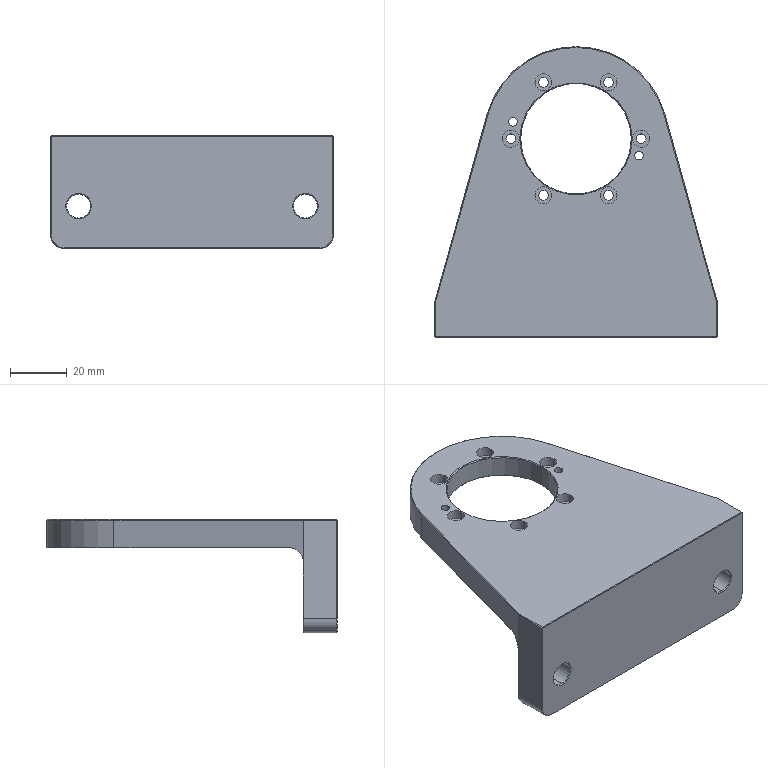NC program | NX | posted with a generic post | part box 100 x 102.5 x 40 mm
Lines 1022 to 2296 of 2296:
(ZLEVEL_PROFILE_1 , TOOL : D6R0.5)
N2006 T16 M6
N2008 G54
N2010 G17 G0 G90 X53.141 Y-17.388 B0. C0. S9500 M3
N2012 G43 Z30. H16
N2014 Z-22.1
N2016 G94 G1 Z-25.1 F3500.
N2018 G3 X50.204 Y-15. R3.
N2020 G1 X-50.204
N2022 X-50.214 Z-25.2
N2024 X50.214
N2026 X50.225 Z-25.3
N2028 X-50.225
N2030 X-50.236 Y-15.001 Z-25.4
N2032 X50.236
N2034 X50.247 Y-15.002 Z-25.5
N2036 X-50.247
N2038 X-50.258 Y-15.004 Z-25.6
N2040 X-49.999 Y-15.001
N2042 X49.999
N2044 X50.258 Y-15.004
N2046 X50.268 Y-15.01 Z-25.7
N2048 X49.998 Y-15.004
N2050 X-49.998
N2052 X-50.268 Y-15.01
N2054 X-50.278 Y-15.016 Z-25.8
N2056 X-49.997 Y-15.01
N2058 X49.997
N2060 X50.278 Y-15.016
N2062 X50.289 Y-15.024 Z-25.899
N2064 X49.994 Y-15.018
N2066 X-49.994
N2068 X-50.289 Y-15.024
N2070 X-50.3 Y-15.031 Z-25.999
N2072 X-49.991 Y-15.028
N2074 X49.991
N2076 X50.3 Y-15.031
N2078 X50.312 Y-15.043 Z-26.098
N2080 X49.987 Y-15.04
N2082 X-49.987
N2084 X-50.312 Y-15.043
N2086 X-50.323 Y-15.059 Z-26.197
N2088 X-49.982 Y-15.054
N2090 X49.982
N2092 X50.323 Y-15.059
N2094 X50.334 Y-15.076 Z-26.296
N2096 X49.978 Y-15.071
N2098 X-49.978
N2100 X-50.334 Y-15.076
N2102 X-50.344 Y-15.095 Z-26.394
N2104 X-49.972 Y-15.09
N2106 X49.972
N2108 X50.344 Y-15.095
N2110 X50.354 Y-15.114 Z-26.492
N2112 X49.965 Y-15.111
N2114 X-49.965
N2116 X-50.354 Y-15.114
N2118 X-50.365 Y-15.137 Z-26.589
N2120 X-49.958 Y-15.134
N2122 X49.958
N2124 X50.365 Y-15.137
N2126 X50.375 Y-15.164 Z-26.686
N2128 X49.95 Y-15.159
N2130 X-49.95
N2132 X-50.375 Y-15.164
N2134 X-50.385 Y-15.191 Z-26.782
N2136 G3 X-49.942 Y-15.186 R21.556
N2138 G1 X49.942
N2140 G3 X50.385 Y-15.191 R4.196
N2142 G1 X50.396 Y-15.221 Z-26.877
N2144 G2 X49.932 Y-15.216 R5.14
N2146 G1 X-49.932
N2148 G2 X-50.396 Y-15.221 R30.468
N2150 G1 X-50.406 Y-15.251 Z-26.972
N2152 X-49.922 Y-15.248
N2154 X49.922
N2156 X50.406 Y-15.251
N2158 X50.405 Y-15.267 Z-27.019
N2160 X50.403 Y-15.285 Z-27.066
N2162 X49.912 Y-15.281
N2164 X-49.912
N2166 X-50.403 Y-15.285
N2168 X-50.39 Y-15.324 Z-27.159
N2170 X-49.901 Y-15.317
N2172 X49.901
N2174 X50.39 Y-15.324
N2176 X50.377 Y-15.362 Z-27.252
N2178 X49.868 Y-15.355
N2180 X-49.868
N2182 X-50.377 Y-15.362
N2184 X-50.364 Y-15.4 Z-27.344
N2186 X-49.877 Y-15.395
N2188 X49.877
N2190 X50.364 Y-15.4
N2192 X50.351 Y-15.438 Z-27.434
N2194 X49.863 Y-15.437
N2196 X-49.863
N2198 X-50.351 Y-15.438
N2200 X-50.345 Y-15.462 Z-27.479
N2202 X-50.339 Y-15.485 Z-27.524
N2204 X-49.85 Y-15.481
N2206 X49.85
N2208 X50.339 Y-15.485
N2210 X50.333 Y-15.508 Z-27.568
N2212 X50.326 Y-15.532 Z-27.613
N2214 X49.836 Y-15.527
N2216 X-49.836
N2218 X-50.326 Y-15.532
N2220 X-50.314 Y-15.578 Z-27.7
N2222 X-49.821 Y-15.575
N2224 X49.821
N2226 X50.314 Y-15.578
N2228 X50.3 Y-15.626 Z-27.787
N2230 X49.847 Y-15.628
N2232 X49.805 Y-15.624
N2234 X-49.805
N2236 X-49.847 Y-15.628
N2238 X-50.3 Y-15.626
N2240 X-50.282 Y-15.68 Z-27.872
N2242 X-49.847 Y-15.682
N2244 X-49.789 Y-15.676
N2246 X49.789
N2248 X49.847 Y-15.682
N2250 X50.283 Y-15.68
N2252 X50.265 Y-15.733 Z-27.957
N2254 X50.193 Y-15.735
N2256 X49.847 Y-15.734
N2258 X49.772 Y-15.73
N2260 X-49.772
N2262 X-49.847 Y-15.734
N2264 X-50.193 Y-15.735
N2266 X-50.265 Y-15.733
N2268 X-50.248 Y-15.786 Z-28.04
N2270 X-50.193 Y-15.788
N2272 X-49.755 Y-15.785
N2274 X49.755
N2276 X50.193 Y-15.788
N2278 X50.248 Y-15.786
N2280 X50.232 Y-15.846 Z-28.122
N2282 X50.193 Y-15.848
N2284 X49.737 Y-15.843
N2286 X-49.737
N2288 X-50.193 Y-15.848
N2290 X-50.232 Y-15.846
N2292 X-50.216 Y-15.905 Z-28.202
N2294 X-49.719 Y-15.902
N2296 X49.719
N2298 X50.216 Y-15.905
N2300 X50.199 Y-15.965 Z-28.281
N2302 X49.7 Y-15.962
N2304 X-49.7
N2306 X-50.199 Y-15.965
N2308 X-50.179 Y-16.032 Z-28.359
N2310 X-49.681 Y-16.025
N2312 X49.681
N2314 X50.179 Y-16.032
N2316 X50.159 Y-16.099 Z-28.436
N2318 X49.661 Y-16.089
N2320 X-49.661
N2322 X-50.158 Y-16.099
N2324 X-50.138 Y-16.164 Z-28.511
N2326 X-49.64 Y-16.155
N2328 X49.64
N2330 X50.138 Y-16.165
N2332 X50.119 Y-16.23 Z-28.584
N2334 X49.619 Y-16.223
N2336 X-49.619
N2338 X-50.119 Y-16.23
N2340 X-50.099 Y-16.295 Z-28.656
N2342 X-49.598 Y-16.292
N2344 X49.598
N2346 X50.099 Y-16.295
N2348 X50.076 Y-16.371 Z-28.726
N2350 X49.575 Y-16.37
N2352 X49.562 Y-16.363
N2354 X-49.562
N2356 X-49.575 Y-16.37
N2358 X-50.076 Y-16.371
N2360 X-50.053 Y-16.446 Z-28.795
N2362 X-49.539 Y-16.435
N2364 X49.539
N2366 X50.053 Y-16.446
N2368 X50.031 Y-16.519 Z-28.862
N2370 X49.516 Y-16.509
N2372 X-49.516
N2374 X-50.031 Y-16.519
N2376 X-50.009 Y-16.591 Z-28.928
N2378 X-49.507 Y-16.584
N2380 X49.507
N2382 X50.009 Y-16.591
N2384 X49.986 Y-16.665 Z-28.991
N2386 X49.483 Y-16.667
N2388 X49.469 Y-16.661
N2390 X-49.469
N2392 X-49.483 Y-16.667
N2394 X-49.986 Y-16.665
N2396 X-49.961 Y-16.748 Z-29.053
N2398 X-49.5 Y-16.75
N2400 X-49.444 Y-16.739
N2402 X49.444
N2404 X49.5 Y-16.75
N2406 X49.961 Y-16.748
N2408 X49.936 Y-16.828 Z-29.114
N2410 X49.5 Y-16.83
N2412 X49.42 Y-16.818
N2414 X-49.42
N2416 X-49.5 Y-16.83
N2418 X-49.936 Y-16.828
N2420 X-49.913 Y-16.907 Z-29.172
N2422 X-49.394 Y-16.899
N2424 X49.394
N2426 X49.913 Y-16.907
N2428 X49.89 Y-16.984 Z-29.229
N2430 X49.383 Y-16.981
N2432 X-49.383
N2434 X-49.89 Y-16.984
N2436 X-49.864 Y-17.069 Z-29.284
N2438 X-49.34 Y-17.064
N2440 X49.34
N2442 X49.864 Y-17.069
N2444 X49.838 Y-17.155 Z-29.336
N2446 X49.314 Y-17.148
N2448 X-49.314
N2450 X-49.838 Y-17.155
N2452 X-49.811 Y-17.242 Z-29.388
N2454 X-49.287 Y-17.233
N2456 X49.287
N2458 X49.811 Y-17.242
N2460 X49.785 Y-17.326 Z-29.437
N2462 X49.294 Y-17.325
N2464 X49.278 Y-17.32
N2466 X-49.278
N2468 X-49.295 Y-17.325
N2470 X-49.785 Y-17.326
N2472 X-49.757 Y-17.419 Z-29.484
N2474 X-49.242 Y-17.407
N2476 X49.242
N2478 X49.757 Y-17.419
N2480 X49.729 Y-17.509 Z-29.529
N2482 X49.214 Y-17.496
N2484 X-49.214
N2486 X-49.729 Y-17.509
N2488 X-49.703 Y-17.594 Z-29.572
N2490 X-49.186 Y-17.585
N2492 X49.186
N2494 X49.703 Y-17.594
N2496 X49.677 Y-17.678 Z-29.613
N2498 X49.167 Y-17.675
N2500 X-49.167
N2502 X-49.677 Y-17.678
N2504 X-49.647 Y-17.778 Z-29.653
N2506 X-49.139 Y-17.766
N2508 X49.139
N2510 X49.647 Y-17.778
N2512 X49.618 Y-17.872 Z-29.69
N2514 X49.154
N2516 X49.11 Y-17.858
N2518 X-49.11
N2520 X-49.154 Y-17.872
N2522 X-49.618
N2524 X-49.591 Y-17.961 Z-29.725
N2526 X-49.154 Y-17.962
N2528 X-49.082 Y-17.95
N2530 X49.082
N2532 X49.154 Y-17.962
N2534 X49.59
N2536 X49.562 Y-18.054 Z-29.758
N2538 X49.035 Y-18.043
N2540 X-49.035
N2542 X-49.562 Y-18.054
N2544 X-49.533 Y-18.152 Z-29.788
N2546 X-49.005 Y-18.136
N2548 X49.005
N2550 X49.533 Y-18.152
N2552 X49.505 Y-18.243 Z-29.817
N2554 X48.976 Y-18.23
N2556 X-48.976
N2558 X-49.505 Y-18.243
N2560 X-49.477 Y-18.336 Z-29.844
N2562 X-48.947 Y-18.324
N2564 X48.947
N2566 X49.477 Y-18.336
N2568 X49.445 Y-18.439 Z-29.868
N2570 X48.92 Y-18.418
N2572 X-48.92
N2574 X-49.445 Y-18.439
N2576 X-49.414 Y-18.537 Z-29.89
N2578 X-48.891 Y-18.513
N2580 X48.891
N2582 X49.415 Y-18.538
N2584 X49.387 Y-18.627 Z-29.911
N2586 X48.861 Y-18.607
N2588 X-48.861
N2590 X-49.387 Y-18.626
N2592 X-49.361 Y-18.711 Z-29.929
N2594 X-48.848 Y-18.701
N2596 X48.848
N2598 X49.361 Y-18.712
N2600 X49.313 Y-18.868 Z-29.95
N2602 X48.799 Y-18.831
N2604 X-48.799
N2606 X-49.313 Y-18.868
N2608 G3 X-52.015 Y-21.161 R3.
N2610 G1 Z-26.95
N2612 G0 Z30.
(ZLEVEL_PROFILE_1_COPY , TOOL : D6R0.5)
N2614 X49.554 Y3.375
N2616 Z2.995
N2618 G1 Z-0.005
N2620 G3 X47.672 Y0.227 R3.
N2622 G1 X47.734 Y-0.3
N2624 Y-12.
N2626 X47.667 Y-12.512
N2628 X47.776 Y-12.502 Z-0.01
N2630 X47.832 Y-12.
N2632 Y-0.3
N2634 X47.777 Y0.203
N2636 X47.831 Y0.222 Z-0.014
N2638 X47.851 Y0.23 Z-0.017
N2640 X47.858 Y0.197
N2642 X47.934 Y-0.3
N2644 Y-12.
N2646 X47.852 Y-12.525
N2648 X47.913 Y-12.544 Z-0.02
N2650 X47.923 Y-12.547 Z-0.024
N2652 X48.011 Y-12.
N2654 Y-0.3
N2656 X47.918 Y0.255
N2658 X47.977 Y0.277 Z-0.027
N2660 X47.98 Y0.278 Z-0.03
N2662 X48.003 Y0.197
N2664 X48.075 Y-0.3
N2666 Y-12.
N2668 X47.989 Y-12.568
N2670 X48.038 Y-12.583 Z-0.034
N2672 X48.061 Y-12.59 Z-0.037
N2674 X48.138 Y-12.
N2676 Y-0.3
N2678 G3 X48.047 Y0.303 R2.011
N2680 G1 X48.134 Y0.288 Z-0.046
N2682 X48.153 Y0.197
N2684 X48.21 Y-0.3
N2686 Y-12.
N2688 X48.138 Y-12.6
N2690 X48.104 Y-12.71
N2692 X48.223 Y-12.597 Z-0.058
N2694 X48.294 Y-12.
N2696 Y-0.3
N2698 X48.188 Y0.369
N2700 X48.252 Z-0.065
N2702 X48.277 Z-0.072
N2704 X48.388 Y-0.3
N2706 Y-12.
N2708 X48.322 Y-12.559
N2710 X48.427 Y-12.513 Z-0.089
N2712 X48.484 Y-12.
N2714 Y-0.3
N2716 X48.38 Y0.369
N2718 X48.46 Y0.3 Z-0.098
N2720 X48.518 Y0.227 Z-0.107
N2722 X48.58 Y-0.3
N2724 Y-12.
N2726 X48.517 Y-12.532
N2728 X48.607 Y-12.581 Z-0.127
N2730 X48.676 Y-12.
N2732 Y-0.3
N2734 X48.615 Y0.197
N2736 X48.599 Y0.268
N2738 X48.64 Y0.288 Z-0.134
N2740 X48.654 Y0.295 Z-0.141
N2742 X48.679 Y0.197
N2744 X48.738 Y-0.3
N2746 Y-12.
N2748 X48.663 Y-12.613
N2750 X48.7 Y-12.636 Z-0.151
N2752 X48.729 Y-12.654 Z-0.161
N2754 X48.747 Y-12.6
N2756 X48.819 Y-12.
N2758 Y-0.3
N2760 X48.731 Y0.334
N2762 X48.703 Y0.466
N2764 X48.68 Y0.542
N2766 X48.764 Y0.432 Z-0.173
N2768 X48.835 Y0.318 Z-0.185
N2770 X48.861 Y0.197
N2772 X48.914 Y-0.3
N2774 Y-12.
N2776 X48.845 Y-12.6
N2778 X48.839 Y-12.62
N2780 X48.938 Y-12.57 Z-0.211
N2782 X49.009 Y-12.
N2784 Y-0.3
N2786 X48.908 Y0.369
N2788 X48.97 Z-0.225
N2790 X49.002 Z-0.239
N2792 X49.103 Y-0.3
N2794 Y-12.
N2796 X49.037 Y-12.536
N2798 X49.148 Y-12.502 Z-0.268
N2800 X49.164 Y-12.416
N2802 X49.197 Y-12.
N2804 Y-0.3
N2806 X49.101 Y0.369
N2808 X49.178 Y0.286 Z-0.284
N2810 X49.236 Y0.2 Z-0.3
N2812 X49.291 Y-0.3
N2814 Y-12.
N2816 X49.254 Y-12.429
N2818 X49.24 Y-12.509
N2820 X49.282 Y-12.6 Z-0.321
N2822 X49.299 Y-12.523
N2824 X49.351 Y-12.
N2826 Y-0.3
N2828 X49.295 Y0.2
N2830 X49.366 Z-0.347
N2832 X49.422 Y-0.3
N2834 Y-12.
N2836 X49.353 Y-12.601
N2838 X49.399 Z-0.364
N2840 X49.446 Y-12.6 Z-0.382
N2842 X49.514 Y-12.
N2844 Y-0.3
N2846 X49.464 Y0.2
N2848 X49.512 Z-0.4
N2850 X49.554 Z-0.419
N2852 X49.605 Y-0.3
N2854 Y-12.
N2856 X49.559 Y-12.498
N2858 X49.556 Y-12.504
N2860 X49.646 Y-12.5 Z-0.458
N2862 X49.656 Y-12.458
N2864 X49.696 Y-12.
N2866 Y-0.3
N2868 X49.642 Y0.2
N2870 X49.694 Z-0.478
N2872 X49.733 Z-0.498
N2874 X49.786 Y-0.3
N2876 Y-12.
N2878 X49.744 Y-12.475
N2880 X49.737 Y-12.5
N2882 X49.829 Z-0.54
N2884 X49.831 Y-12.491
N2886 X49.876 Y-12.
N2888 Y-0.3
N2890 X49.828 Y0.2
N2892 X49.874 Z-0.561
N2894 X49.914 Z-0.583
N2896 X49.965 Y-0.3
N2898 Y-12.
N2900 X49.92 Y-12.427
N2902 X49.975 Z-0.606
N2904 X50.006 Z-0.628
N2906 X50.053 Y-12.
N2908 Y-0.3
N2910 X49.999 Y0.2
N2912 X50.051 Z-0.652
N2914 X50.088 Z-0.675
N2916 X50.14 Y-0.3
N2918 Y-12.
N2920 X50.095 Y-12.427
N2922 X50.175 Y-12.507 Z-0.723
N2924 X50.193 Y-12.413
N2926 X50.227 Y-12.
N2928 Y-0.3
N2930 X50.18 Y0.2
N2932 X50.223 Y0.205 Z-0.748
N2934 X50.26 Y0.209 Z-0.773
N2936 X50.312 Y-0.3
N2938 Y-12.
N2940 X50.256 Y-12.508
N2942 X50.306 Y-12.515 Z-0.799
N2944 X50.337 Y-12.519 Z-0.825
N2946 X50.397 Y-12.
N2948 Y-0.3
N2950 X50.341 Y0.22
N2952 X50.388 Y0.226 Z-0.851
N2954 X50.424 Y0.231 Z-0.878
N2956 X50.481 Y-0.3
N2958 Y-12.
N2960 X50.42 Y-12.53
N2962 X50.469 Y-12.537 Z-0.905
N2964 X50.505 Y-12.542 Z-0.932
N2966 G3 X50.563 Y-12. R3.656
N2968 G1 Y-0.3
N2970 X50.509 Y0.242
N2972 X50.55 Y0.241 Z-0.959
N2974 X50.589 Y0.24 Z-0.987
N2976 X50.644 Y-0.3
N2978 Y-12.
N2980 X50.584 Y-12.539
N2982 X50.632 Y-12.533 Z-1.016
N2984 X50.664 Y-12.529 Z-1.044
N2986 X50.725 Y-12.
N2988 Y-0.3
N2990 X50.669 Y0.229
N2992 X50.75 Y0.218 Z-1.103
N2994 X50.804 Y-0.3
N2996 Y-12.
N2998 X50.746 Y-12.517
N3000 X50.797 Y-12.51 Z-1.134
N3002 X50.829 Y-12.506 Z-1.164
N3004 G3 X50.883 Y-12. R3.548
N3006 G1 Y-0.3
N3008 X50.834 Y0.207
N3010 X50.914 Y0.2 Z-1.226
N3012 X50.961 Y-0.3
N3014 Y-12.
N3016 X50.91 Y-12.499
N3018 X50.955 Z-1.257
N3020 X50.983 Z-1.289
N3022 X51.038 Y-12.
N3024 Y-0.3
N3026 X50.987 Y0.2
N3028 X51.031 Z-1.321
N3030 X51.062 Z-1.354
N3032 X51.113 Y-0.3
N3034 Y-12.
N3036 X51.057 Y-12.499
N3038 X51.106 Z-1.387
N3040 X51.133 Z-1.42
N3042 G3 X51.188 Y-12. R3.177
N3044 G1 Y-0.3
N3046 X51.138 Y0.2
N3048 X51.18 Z-1.453
N3050 X51.216 Z-1.487
N3052 X51.261 Y-0.3
N3054 Y-12.
N3056 G2 X51.212 Y-12.499 R2.867
N3058 G1 X51.253 Z-1.521
N3060 X51.281 Z-1.556
N3062 X51.333 Y-12.
N3064 Y-0.3
N3066 X51.285 Y0.2
N3068 X51.324 Z-1.591
N3070 X51.353 Z-1.626
N3072 X51.404 Y-0.3
N3074 Y-12.
N3076 X51.35 Y-12.5
N3078 X51.394 Z-1.661
N3080 X51.42 Z-1.697
N3082 X51.473 Y-12.
N3084 Y-0.3
N3086 X51.422 Y0.2
N3088 X51.463 Z-1.733
N3090 X51.492 Z-1.77
N3092 X51.542 Y-0.3
N3094 Y-12.
N3096 G2 X51.492 Y-12.5 R3.594
N3098 G1 X51.531 Z-1.806
N3100 X51.564 Z-1.843
N3102 X51.577 Y-12.404
N3104 X51.608 Y-12.
N3106 Y-0.3
N3108 X51.564 Y0.2
N3110 X51.597 Z-1.881
N3112 X51.626 Z-1.918
N3114 X51.674 Y-0.3
N3116 Y-12.
N3118 X51.627 Y-12.5
N3120 X51.662 Z-1.957
N3122 X51.688 Z-1.995
N3124 X51.738 Y-12.
N3126 Y-0.3
N3128 X51.687 Y0.2
N3130 X51.726 Z-2.033
N3132 X51.749 Z-2.072
N3134 X51.801 Y-0.3
N3136 Y-12.
N3138 X51.749 Y-12.5
N3140 X51.789 Z-2.111
N3142 X51.812 Z-2.151
N3144 G3 X51.863 Y-12. R3.703
N3146 G1 Y-0.3
N3148 X51.812 Y0.2
N3150 X51.849 Z-2.19
N3152 X51.875 Z-2.23
N3154 G2 X51.923 Y-0.3 R5.272
N3156 G1 Y-12.
N3158 G2 X51.875 Y-12.5 R3.552
N3160 G1 X51.909 Z-2.271
N3162 X51.937 Z-2.311
N3164 G3 X51.981 Y-12. R4.011
N3166 G1 Y-0.3
N3168 G3 X51.937 Y0.2 R5.865
N3170 G1 X51.967 Z-2.352
N3172 X51.993 Z-2.393
N3174 G2 X52.038 Y-0.3 R5.372
N3176 G1 Y-12.
N3178 G2 X51.996 Y-12.501 R4.747
N3180 G1 X52.023 Z-2.434
N3182 X52.052 Z-2.476
N3184 G3 X52.094 Y-12. R4.38
N3186 G1 Y-0.3
N3188 G3 X52.049 Y0.201 R4.749
N3190 G1 X52.077 Z-2.518
N3192 X52.104 Z-2.56
N3194 G2 X52.148 Y-0.3 R4.373
N3196 G1 Y-12.
N3198 G2 X52.103 Y-12.501 R4.438
N3200 G1 X52.131 Z-2.602
N3202 X52.154 Z-2.644
N3204 G3 X52.201 Y-12. R4.542
N3206 G1 Y-0.3
N3208 G3 X52.155 Y0.201 R4.671
N3210 G1 X52.183 Z-2.687
N3212 X52.206 Y0.2 Z-2.73
N3214 G2 X52.252 Y-0.3 R5.016
N3216 G1 Y-12.
N3218 G2 X52.207 Y-12.501 R3.849
N3220 G1 X52.233 Y-12.5 Z-2.773
N3222 X52.258 Z-2.817
N3224 G3 X52.301 Y-12. R4.005
N3226 G1 Y-0.3
N3228 G3 X52.258 Y0.2 R5.42
N3230 G1 X52.282 Z-2.861
N3232 X52.304 Z-2.904
N3234 G2 X52.349 Y-0.3 R6.652
N3236 G1 Y-12.
N3238 G2 X52.307 Y-12.501 R4.563
N3240 G1 X52.33 Z-2.949
N3242 X52.356 Z-2.993
N3244 G3 X52.395 Y-12. R4.798
N3246 G1 Y-0.3
N3248 G3 X52.349 Y0.201 R6.111
N3250 G1 X52.375 Z-3.038
N3252 X52.395 Z-3.082
N3254 G2 X52.44 Y-0.3 R5.647
N3256 G1 Y-12.
N3258 G2 X52.399 Y-12.502 R4.675
N3260 G1 X52.418 Z-3.127
N3262 X52.44 Z-3.172
N3264 G3 X52.483 Y-12. R4.85
N3266 G1 Y-0.3
N3268 G3 X52.44 Y0.202 R5.245
N3270 G1 X52.461 Y0.201 Z-3.218
N3272 X52.479 Z-3.263
N3274 G2 X52.525 Y-0.3 R6.023
N3276 G1 Y-12.
N3278 G2 X52.48 Y-12.502 R4.294
N3280 G1 X52.501 Z-3.309
N3282 X52.52 Y-12.501 Z-3.355
N3284 G3 X52.564 Y-12. R4.318
N3286 G1 Y-0.3
N3288 G3 X52.517 Y0.201 R6.021
N3290 G1 X52.54 Z-3.401
N3292 X52.556 Y0.2 Z-3.447
N3294 G2 X52.603 Y-0.3 R6.017
N3296 G1 Y-12.
N3298 G2 X52.56 Y-12.501 R4.34
N3300 G1 X52.578 Z-3.494
N3302 X52.6 Z-3.54
N3304 G3 X52.639 Y-12. R5.108
N3306 G1 Y-0.3
N3308 G3 X52.595 Y0.2 R6.011
N3310 G1 X52.615 Z-3.587
N3312 X52.63 Z-3.634
N3314 X52.674 Y-0.3
N3316 Y-12.
N3318 X52.635 Y-12.501
N3320 X52.647 Z-3.681
N3322 X52.666 Z-3.728
N3324 X52.707 Y-12.
N3326 Y-0.3
N3328 X52.659 Y0.201
N3330 X52.679 Z-3.776
N3332 X52.689 Z-3.823
N3334 X52.738 Y-0.3
N3336 Y-12.
N3338 X52.696 Y-12.502
N3340 X52.709 Y-12.503 Z-3.871
N3342 X52.727 Z-3.919
N3344 X52.768 Y-12.
N3346 Y-0.3
N3348 G3 X52.719 Y0.202 R7.437
N3350 G1 X52.738 Z-3.967
N3352 X52.749 Z-4.015
N3354 G2 X52.796 Y-0.3 R2.742
N3356 G1 Y-12.
N3358 G2 X52.758 Y-12.504 R4.852
N3360 G1 X52.766 Z-4.063
N3362 X52.787 Z-4.111
N3364 X52.822 Y-12.
N3366 Y-0.3
N3368 G3 X52.779 Y0.203 R7.05
N3370 G1 X52.791 Z-4.16
N3372 X52.803 Y0.202 Z-4.208
N3374 G2 X52.846 Y-0.3 R9.347
N3376 G1 Y-12.
N3378 X52.811 Y-12.504
N3380 X52.817 Z-4.257
N3382 X52.833 Z-4.306
N3384 X52.869 Y-12.
N3386 Y-0.3
N3388 G3 X52.824 Y0.202 R3.267
N3390 G1 X52.837 Z-4.354
N3392 X52.845 Z-4.403
N3394 G2 X52.89 Y-0.3 R8.797
N3396 G1 Y-12.
N3398 G2 X52.856 Y-12.504 R5.535
N3400 G1 X52.86 Z-4.452
N3402 X52.876 Y-12.503 Z-4.501
N3404 X52.909 Y-12.
N3406 Y-0.3
N3408 X52.866 Y0.202
N3410 X52.876 Z-4.551
N3412 X52.884 Z-4.6
N3414 X52.926 Y-0.3
N3416 Y-12.
N3418 X52.897 Y-12.503
N3420 X52.902 Y-12.502 Z-4.649
N3422 X52.916 Z-4.699
N3424 X52.941 Y-12.
N3426 Y-0.3
N3428 X52.901 Y0.201
N3430 X52.913 Z-4.748
N3432 X52.918 Z-4.798
N3434 X52.955 Y-0.3
N3436 Y-12.
N3438 X52.932 Y-12.501
N3440 X52.941 Z-4.847
N3442 X52.946 Y-12.5 Z-4.897
N3444 X52.967 Y-12.
N3446 Y-0.3
N3448 G3 X52.935 Y0.2 R10.725
N3450 G1 X52.948 Z-4.947
N3452 X52.952 Z-4.997
N3454 X52.977 Y-0.3
N3456 Y-12.
N3458 X52.958 Y-12.5
N3460 X52.965 Z-5.046
N3462 X52.969 Z-5.096
N3464 X52.985 Y-12.
N3466 Y-0.3
N3468 X52.966 Y0.2
N3470 X52.975 Y0.201 Z-5.196
N3472 X52.992 Y-0.3
N3474 Y-12.
N3476 X52.977 Y-12.5
N3478 X52.983 Z-5.272
N3480 X52.995 Y-12.
N3482 Y-0.3
N3484 X52.982 Y0.201
N3486 X52.988 Z-5.348
N3488 X52.998 Y-0.3
N3490 Y-12.
N3492 X52.989 Y-12.5
N3494 X52.995 Z-5.424
N3496 X52.998 Y-12.
N3498 Y-0.3
N3500 X52.995 Y0.202
N3502 X52.997 Z-5.5
N3504 X52.999 Y-0.495
N3506 Y-11.909
N3508 X52.996 Y-12.5
N3510 G3 X55.244 Y-15.416 R3.
N3512 G1 Z-2.5
N3514 G0 Z30.
N3516 X-49.553 Y-15.71
N3518 Z2.995
N3520 G1 Z-0.005
N3522 G3 X-47.665 Y-12.511 R3.
N3524 G1 X-47.734 Y-12.
N3526 Y-0.3
N3528 X-47.666 Y0.212
N3530 X-47.724 Y0.219 Z-0.008
N3532 X-47.774 Y0.225 Z-0.01
N3534 X-47.832 Y-0.3
N3536 Y-12.
N3538 X-47.785 Y-12.438
N3540 X-47.776 Y-12.502
N3542 X-47.832 Y-12.519 Z-0.014
N3544 X-47.852 Y-12.525 Z-0.017
N3546 X-47.934 Y-12.
N3548 Y-0.3
N3550 X-47.821 Y0.369
N3552 X-47.89 Z-0.024
N3554 X-48.011 Y-0.3
N3556 Y-12.
N3558 X-47.923 Y-12.547
N3560 X-47.979 Y-12.565 Z-0.027
N3562 X-47.989 Y-12.568 Z-0.03
N3564 X-48.075 Y-12.
N3566 Y-0.3
N3568 X-47.955 Y0.369
N3570 X-48.026 Z-0.037
N3572 G3 X-48.138 Y-0.3 R1.873
N3574 G1 Y-12.
N3576 X-48.061 Y-12.59
N3578 X-48.145 Y-12.575 Z-0.046
N3580 X-48.154 Y-12.533
N3582 X-48.21 Y-12.
N3584 Y-0.3
N3586 X-48.086 Y0.455
N3588 X-48.17 Y0.441 Z-0.058
N3590 X-48.294 Y-0.3
N3592 Y-12.
N3594 X-48.235 Y-12.521
N3596 X-48.332 Y-12.476 Z-0.072
N3598 X-48.388 Y-12.
N3600 Y-0.3
N3602 X-48.284 Y0.343
N3604 X-48.365 Y0.289 Z-0.08
N3606 X-48.42 Y0.232 Z-0.089
N3608 X-48.484 Y-0.3
N3610 Y-12.
N3612 X-48.439 Y-12.46
N3614 X-48.432 Y-12.496
N3616 X-48.517 Y-12.532 Z-0.107
N3618 X-48.58 Y-12.
N3620 Y-0.3
N3622 X-48.517 Y0.231
N3624 X-48.597 Y0.278 Z-0.127
N3626 X-48.615 Y0.197
N3628 X-48.676 Y-0.3
N3630 Y-12.
N3632 X-48.607 Y-12.581
N3634 X-48.664 Y-12.61 Z-0.141
N3636 X-48.738 Y-12.
N3638 Y-0.3
N3640 X-48.679 Y0.197
N3642 X-48.651 Y0.309
N3644 X-48.675 Y0.429 Z-0.151
N3646 X-48.679 Y0.542 Z-0.161
N3648 X-48.703 Y0.466
N3650 X-48.726 Y0.353
N3652 X-48.819 Y-0.3
N3654 Y-12.
N3656 X-48.747 Y-12.6
N3658 X-48.734 Y-12.64
N3660 X-48.842 Y-12.61 Z-0.185
N3662 X-48.845 Y-12.6
N3664 X-48.914 Y-12.
N3666 Y-0.3
N3668 X-48.818 Y0.395
N3670 X-48.917 Y0.334 Z-0.211
N3672 X-49.009 Y-0.3
N3674 Y-12.
N3676 X-48.96 Y-12.427
N3678 X-49.021 Z-0.225
N3680 X-49.056 Z-0.239
N3682 X-49.103 Y-12.
N3684 Y-0.3
N3686 X-49.048 Y0.197
N3688 X-49.028 Y0.27
N3690 X-49.148 Y0.203 Z-0.268
N3692 X-49.197 Y-0.3
N3694 Y-12.
N3696 X-49.154 Y-12.476
N3698 X-49.14 Y-12.538
N3700 X-49.24 Y-12.509 Z-0.3
N3702 X-49.254 Y-12.429
N3704 X-49.291 Y-12.
N3706 Y-0.3
N3708 X-49.236 Y0.2
N3710 X-49.273 Z-0.31
N3712 X-49.295 Z-0.321
N3714 X-49.351 Y-0.3
N3716 Y-12.
N3718 X-49.299 Y-12.523
N3720 X-49.282 Y-12.6
N3722 X-49.353 Y-12.601 Z-0.347
N3724 X-49.422 Y-12.
N3726 Y-0.3
N3728 X-49.366 Y0.2
N3730 X-49.421 Z-0.364
N3732 X-49.464 Z-0.382
N3734 X-49.514 Y-0.3
N3736 Y-12.
N3738 X-49.446 Y-12.6
N3740 X-49.51 Y-12.515 Z-0.4
N3742 X-49.561 Y-12.427 Z-0.419
N3744 X-49.605 Y-12.
N3746 Y-0.3
N3748 X-49.554 Y0.2
N3750 X-49.604 Z-0.438
N3752 X-49.642 Z-0.458
N3754 X-49.696 Y-0.3
N3756 Y-12.
N3758 X-49.649 Y-12.427
N3760 X-49.707 Z-0.478
N3762 X-49.74 Z-0.498
N3764 X-49.786 Y-12.
N3766 Y-0.3
N3768 X-49.733 Y0.2
N3770 X-49.784 Z-0.519
N3772 X-49.828 Z-0.54
N3774 X-49.876 Y-0.3
N3776 Y-12.
N3778 X-49.826 Y-12.49
N3780 X-49.875 Y-12.495 Z-0.561
N3782 X-49.909 Y-12.499 Z-0.583
N3784 X-49.965 Y-12.
N3786 Y-0.3
N3788 X-49.914 Y0.2
N3790 X-49.962 Z-0.606
N3792 X-49.999 Z-0.628
N3794 X-50.053 Y-0.3
N3796 Y-12.
N3798 X-49.995 Y-12.499
N3800 X-50.05 Z-0.652
N3802 X-50.083 Z-0.675
N3804 X-50.14 Y-12.
N3806 Y-0.3
N3808 X-50.088 Y0.2
N3810 X-50.138 Z-0.699
N3812 X-50.18 Z-0.723
N3814 X-50.227 Y-0.3
N3816 Y-12.
N3818 X-50.193 Y-12.413
N3820 X-50.177 Y-12.499
N3822 X-50.223 Y-12.505 Z-0.748
N3824 X-50.256 Y-12.508 Z-0.773
N3826 X-50.312 Y-12.
N3828 Y-0.3
N3830 X-50.26 Y0.209
N3832 X-50.306 Y0.215 Z-0.799
N3834 X-50.341 Y0.22 Z-0.825
N3836 X-50.397 Y-0.3
N3838 Y-12.
N3840 X-50.337 Y-12.519
N3842 X-50.388 Y-12.526 Z-0.851
N3844 X-50.42 Y-12.53 Z-0.878
N3846 X-50.481 Y-12.
N3848 Y-0.3
N3850 X-50.424 Y0.231
N3852 X-50.469 Y0.237 Z-0.905
N3854 X-50.509 Y0.242 Z-0.932
N3856 X-50.563 Y-0.3
N3858 Y-12.
N3860 G3 X-50.505 Y-12.542 R9.321
N3862 G1 X-50.55 Y-12.54 Z-0.959
N3864 X-50.584 Y-12.539 Z-0.987
N3866 X-50.644 Y-12.
N3868 Y-0.3
N3870 X-50.589 Y0.24
N3872 X-50.632 Y0.234 Z-1.016
N3874 X-50.669 Y0.229 Z-1.044
N3876 X-50.725 Y-0.3
N3878 Y-12.
N3880 X-50.664 Y-12.528
N3882 X-50.715 Y-12.521 Z-1.074
N3884 X-50.746 Y-12.517 Z-1.103
N3886 X-50.804 Y-12.
N3888 Y-0.3
N3890 X-50.75 Y0.218
N3892 X-50.834 Y0.207 Z-1.164
N3894 X-50.883 Y-0.3
N3896 Y-12.
N3898 G3 X-50.829 Y-12.506 R12.104
N3900 G1 X-50.877 Y-12.502 Z-1.195
N3902 X-50.91 Y-12.499 Z-1.226
N3904 X-50.961 Y-12.
N3906 Y-0.3
N3908 X-50.914 Y0.2
N3910 X-50.955 Z-1.257
N3912 X-50.987 Z-1.289
N3914 X-51.038 Y-0.3
N3916 Y-12.
N3918 X-50.983 Y-12.499
N3920 X-51.031 Z-1.321
N3922 X-51.057 Z-1.354
N3924 X-51.113 Y-12.
N3926 Y-0.3
N3928 X-51.062 Y0.2
N3930 X-51.106 Z-1.387
N3932 X-51.138 Z-1.42
N3934 X-51.188 Y-0.3
N3936 Y-12.
N3938 G3 X-51.133 Y-12.499 R4.952
N3940 G1 X-51.18 Z-1.453
N3942 X-51.212 Z-1.487
N3944 G2 X-51.261 Y-12. R2.867
N3946 G1 Y-0.3
N3948 X-51.216 Y0.2
N3950 X-51.252 Z-1.521
N3952 X-51.285 Z-1.556
N3954 X-51.333 Y-0.3
N3956 Y-12.
N3958 X-51.281 Y-12.499
N3960 X-51.324 Y-12.5 Z-1.591
N3962 X-51.35 Z-1.626
N3964 X-51.404 Y-12.
N3966 Y-0.3
N3968 X-51.353 Y0.2
N3970 X-51.394 Z-1.661
N3972 X-51.422 Z-1.697
N3974 X-51.473 Y-0.3
N3976 Y-12.
N3978 X-51.42 Y-12.5
N3980 X-51.463 Z-1.733
N3982 X-51.492 Z-1.77
N3984 G2 X-51.542 Y-12. R19.188
N3986 G1 Y-0.3
N3988 X-51.492 Y0.2
N3990 X-51.531 Z-1.806
N3992 X-51.564 Z-1.843
N3994 X-51.608 Y-0.3
N3996 Y-12.
N3998 X-51.577 Y-12.404
N4000 X-51.564 Y-12.5
N4002 X-51.597 Z-1.881
N4004 X-51.627 Z-1.918
N4006 X-51.674 Y-12.
N4008 Y-0.3
N4010 X-51.626 Y0.2
N4012 X-51.662 Z-1.957
N4014 X-51.687 Z-1.995
N4016 X-51.738 Y-0.3
N4018 Y-12.
N4020 X-51.688 Y-12.5
N4022 X-51.726 Z-2.033
N4024 X-51.749 Z-2.072
N4026 X-51.801 Y-12.
N4028 Y-0.3
N4030 X-51.749 Y0.2
N4032 X-51.788 Z-2.111
N4034 X-51.812 Z-2.151
N4036 X-51.863 Y-0.3
N4038 Y-12.
N4040 G3 X-51.812 Y-12.5 R3.703
N4042 G1 X-51.849 Z-2.19
N4044 X-51.875 Z-2.23
N4046 G2 X-51.923 Y-12. R3.552
N4048 G1 Y-0.3
N4050 G2 X-51.875 Y0.2 R5.272
N4052 G1 X-51.909 Z-2.271
N4054 X-51.937 Z-2.311
N4056 G3 X-51.981 Y-0.3 R5.483
N4058 G1 Y-12.
N4060 G3 X-51.937 Y-12.5 R3.409
N4062 G1 X-51.967 Z-2.352
N4064 X-51.996 Y-12.501 Z-2.393
N4066 G2 X-52.038 Y-12. R4.401
N4068 G1 Y-0.3
N4070 G2 X-51.993 Y0.2 R5.372
N4072 G1 X-52.023 Y0.201 Z-2.434
N4074 X-52.049 Z-2.476
N4076 G3 X-52.094 Y-0.3 R4.749
N4078 G1 Y-12.
N4080 G3 X-52.052 Y-12.501 R6.692
N4082 G1 X-52.077 Z-2.518
N4084 X-52.103 Z-2.56
N4086 G2 X-52.148 Y-12. R7.244
N4088 G1 Y-0.3
N4090 G2 X-52.104 Y0.201 R4.373
N4092 G1 X-52.131 Z-2.602
N4094 X-52.155 Z-2.644
N4096 G3 X-52.201 Y-0.3 R4.671
N4098 G1 Y-12.
N4100 G3 X-52.154 Y-12.501 R4.542
N4102 G1 X-52.183 Z-2.687
N4104 X-52.207 Z-2.73
N4106 G2 X-52.252 Y-12. R3.124
N4108 G1 Y-0.3
N4110 G2 X-52.206 Y0.2 R5.016
N4112 G1 X-52.234 Z-2.773
N4114 X-52.258 Z-2.817
N4116 G3 X-52.301 Y-0.3 R5.42
N4118 G1 Y-12.
N4120 G3 X-52.258 Y-12.5 R3.627
N4122 G1 X-52.282 Z-2.861
N4124 X-52.307 Y-12.501 Z-2.904
N4126 G2 X-52.349 Y-12. R4.563
N4128 G1 Y-0.3
N4130 G2 X-52.304 Y0.2 R6.652
N4132 G1 X-52.33 Z-2.949
N4134 X-52.349 Y0.201 Z-2.993
N4136 G3 X-52.395 Y-0.3 R6.111
N4138 G1 Y-12.
N4140 G3 X-52.356 Y-12.501 R4.798
N4142 G1 X-52.374 Y-12.502 Z-3.038
N4144 X-52.399 Z-3.082
N4146 G2 X-52.44 Y-12. R8.02
N4148 G1 Y-0.3
N4150 G2 X-52.395 Y0.201 R5.647
N4152 G1 X-52.418 Z-3.127
N4154 X-52.44 Y0.202 Z-3.172
N4156 G3 X-52.483 Y-0.3 R5.245
N4158 G1 Y-12.
N4160 G3 X-52.44 Y-12.502 R8.76
N4162 G1 X-52.461 Z-3.218
N4164 X-52.48 Z-3.263
N4166 G2 X-52.525 Y-12. R9.043
N4168 G1 Y-0.3
N4170 G2 X-52.479 Y0.201 R6.03
N4172 G1 X-52.501 Z-3.309
N4174 X-52.517 Z-3.355
N4176 G3 X-52.564 Y-0.3 R6.051
N4178 G1 Y-12.
N4180 G3 X-52.52 Y-12.501 R5.368
N4182 G1 X-52.54 Z-3.401
N4184 X-52.56 Z-3.447
N4186 G2 X-52.603 Y-12. R5.525
N4188 G1 Y-0.3
N4190 G2 X-52.556 Y0.2 R6.07
N4192 G1 X-52.578 Z-3.494
N4194 X-52.595 Z-3.54
N4196 G3 X-52.639 Y-0.3 R6.087
N4198 G1 Y-12.
N4200 G3 X-52.6 Y-12.501 R5.089
N4202 G1 X-52.614 Z-3.587
N4204 X-52.635 Z-3.634
N4206 X-52.674 Y-12.
N4208 Y-0.3
N4210 X-52.63 Y0.2
N4212 X-52.647 Z-3.681
N4214 X-52.66 Y0.201 Z-3.728
N4216 X-52.707 Y-0.3
N4218 Y-12.
N4220 X-52.665 Y-12.502
N4222 X-52.679 Z-3.776
N4224 X-52.696 Z-3.823
N4226 X-52.738 Y-12.
N4228 Y-0.3
N4230 X-52.69 Y0.201
N4232 X-52.71 Z-3.871
N4234 X-52.72 Y0.202 Z-3.919
N4236 G3 X-52.768 Y-0.3 R7.841
N4238 G1 Y-12.
N4240 G3 X-52.726 Y-12.503 R8.865
N4242 G1 X-52.738 Y-12.504 Z-3.967
N4244 X-52.756 Z-4.015
N4246 G2 X-52.796 Y-12. R7.511
N4248 G1 Y-0.3
N4250 G2 X-52.75 Y0.202 R2.844
N4252 G1 X-52.766 Z-4.063
N4254 X-52.781 Y0.203 Z-4.111
N4256 G3 X-52.822 Y-0.3 R7.66
N4258 G1 Y-12.
N4260 G3 X-52.785 Y-12.504 R7.316
N4262 G1 X-52.791 Z-4.16
N4264 X-52.809 Z-4.208
N4266 X-52.846 Y-12.
N4268 Y-0.3
N4270 G2 X-52.805 Y0.202 R10.746
N4272 G1 X-52.816 Z-4.257
N4274 X-52.826 Z-4.306
N4276 G3 X-52.869 Y-0.3 R10.083
N4278 G1 Y-12.
N4280 G3 X-52.831 Y-12.504 R5.776
N4282 G1 X-52.837 Y-12.505 Z-4.354
N4284 X-52.852 Z-4.403
N4286 G2 X-52.89 Y-12. R5.553
N4288 G1 Y-0.3
N4290 G2 X-52.848 Y0.202 R9.492
N4292 G1 X-52.86 Z-4.452
N4294 X-52.87 Z-4.501
N4296 X-52.909 Y-0.3
N4298 Y-12.
N4300 G3 X-52.872 Y-12.504 R5.509
N4302 G1 X-52.876 Z-4.551
N4304 X-52.892 Y-12.503 Z-4.6
N4306 G2 X-52.926 Y-12. R5.501
N4308 G1 Y-0.3
N4310 X-52.891 Y0.202
N4312 X-52.902 Z-4.649
N4314 X-52.912 Z-4.699
N4316 X-52.941 Y-0.3
N4318 Y-12.
N4320 X-52.91 Y-12.502
N4322 X-52.913 Z-4.748
N4324 X-52.927 Y-12.501 Z-4.798
N4326 X-52.955 Y-12.
N4328 Y-0.3
N4330 X-52.929 Y0.201
N4332 X-52.941 Z-4.847
N4334 X-52.944 Z-4.897
N4336 X-52.967 Y-0.3
N4338 Y-12.
N4340 X-52.941 Y-12.501
N4342 X-52.948 Z-4.947
N4344 X-52.955 Y-12.5 Z-4.997
N4346 X-52.977 Y-12.
N4348 Y-0.3
N4350 X-52.958 Y0.2
N4352 X-52.968 Z-5.096
N4354 X-52.985 Y-0.3
N4356 Y-12.
N4358 X-52.966 Y-12.5
N4360 X-52.975 Z-5.196
N4362 X-52.992 Y-12.
N4364 Y-0.3
N4366 G3 X-52.977 Y0.201 R4.836
N4368 G1 X-52.983 Z-5.272
N4370 G2 X-52.995 Y-0.3 R5.173
N4372 G1 Y-12.
N4374 X-52.982 Y-12.5
N4376 X-52.988 Z-5.348
N4378 X-52.998 Y-12.
N4380 Y-0.3
N4382 X-52.989 Y0.201
N4384 X-52.995 Y0.202 Z-5.424
N4386 X-52.999 Y-0.3
N4388 Y-12.
N4390 X-52.995 Y-12.5
N4392 X-52.998 Z-5.5
N4394 X-52.999 Y-12.
N4396 X-53. Y-0.495
N4398 X-52.997 Y0.202
N4400 G3 X-55.244 Y3.117 R3.
N4402 G1 Z-2.5
N4404 G0 Z30.
N4406 M5
(PLANAR_MILL_COPY_COPY_COPY_COPY_COPY_COPY_1_COPY_1_COPY , TOOL : D6A45)
N4408 T01 M6
N4410 G54
N4412 G17 G0 G90 X0.866 Y-13.3 B0. C0. S9500 M3
N4414 G43 Z30. H1
N4416 Z0.5
N4418 G94 G1 Z-1. F1250.
N4420 G3 X0. Y-12.8 R1.
N4422 G1 X-50.
N4424 G2 X-50.8 Y-12. R0.8
N4426 G1 Y-0.3
N4428 G2 X-50.566 Y0.266 R0.8
N4430 G1 X-50.266 Y0.566
N4432 G2 X-49.7 Y0.8 R0.8
N4434 G1 X49.7
N4436 G2 X50.266 Y0.566 R0.8
N4438 G1 X50.566 Y0.266
N4440 G2 X50.8 Y-0.3 R0.8
N4442 G1 Y-12.
N4444 G2 X50. Y-12.8 R0.8
N4446 G1 X0.
N4448 G3 X-0.866 Y-13.3 R1.
N4450 G1 Z0.5
N4452 G0 Z30.
(PLANAR_MILL_COPY_COPY_COPY_COPY_COPY_COPY_1_COPY_1_COPY_COPY , TOOL : D6A45)
N4454 X49.651 Y-21.581
N4456 Z-29.5
N4458 G1 Z-31.
N4460 X49.316 Y-21.
N4462 G3 X48.45 Y-20.5 R1.
N4464 G1 X32.065 Y-78.983
N4466 G2 X-32.065 Y-78.983 R33.3
N4468 G1 X-48.45 Y-20.5
N4470 G3 X-49.316 Y-21. R1.
N4472 G1 X-49.651 Y-21.581
N4474 Z-29.5
N4476 G0 Z30.
N4478 X-1.291 Y-93.565
N4480 Z-29.5
N4482 G1 Z-31.
N4484 X-0.866 Y-94.3
N4486 G3 X0. Y-94.8 R1.
N4488 X24.8 Y-70. R24.8
N4490 X0. Y-94.8 R-24.8
N4492 X0.866 Y-94.3 R1.
N4494 G1 X1.291 Y-93.565
N4496 Z-29.5
N4498 G0 Z30.
(PLANAR_MILL_COPY_COPY_COPY_COPY_COPY_COPY_1_COPY_1_COPY_COPY_COPY , TOOL : D6A)
N4500 X-17.452 Y-68.702
N4502 Z-31.5
N4504 G1 Z-33.
N4506 X-18.2 Y-69.134
N4508 G3 X-18.7 Y-70. R1.
N4510 X0. Y-88.7 R18.7
N4512 X-18.7 Y-70. R-18.7
N4514 X-18.2 Y-70.866 R1.
N4516 G1 X-17.452 Y-71.298
N4518 Z-31.5
N4520 G0 Z30.
N4522 M5
N4524 M2